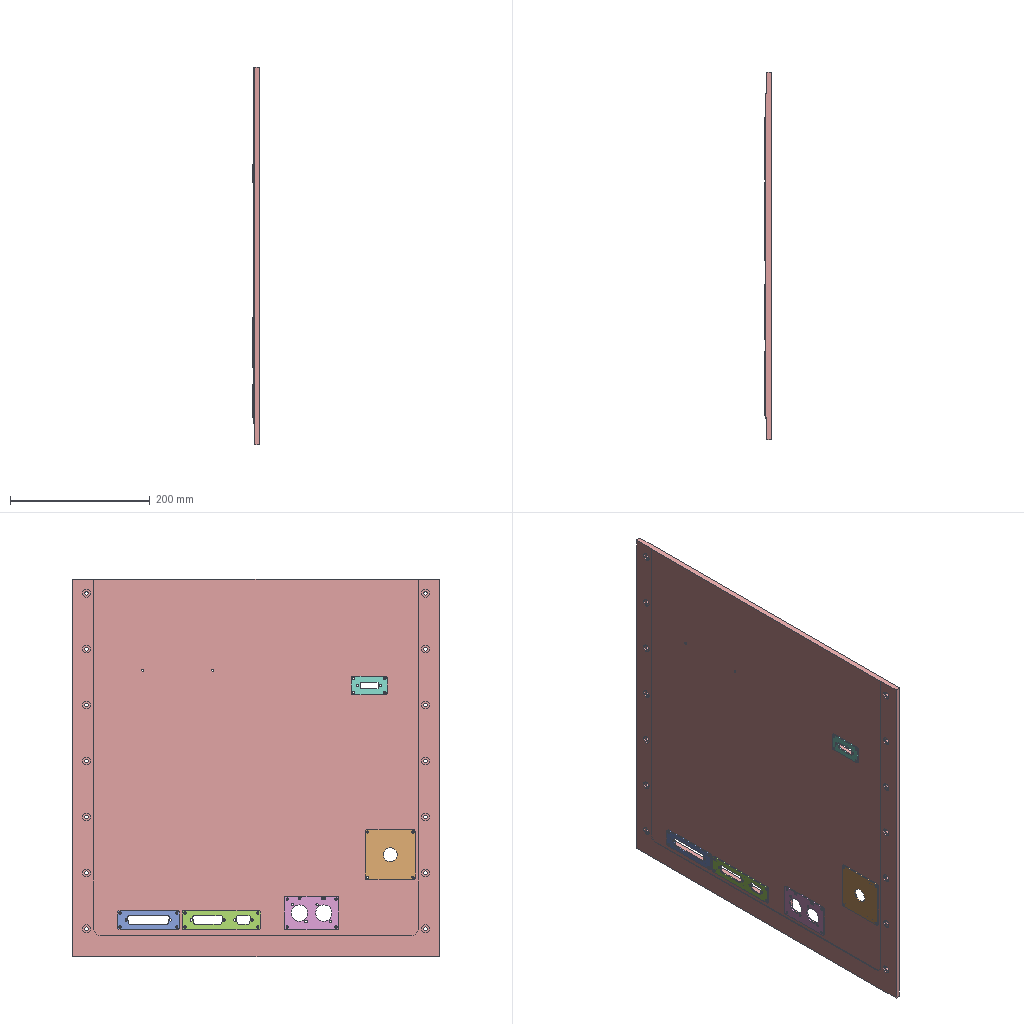Assembly | SolidWorks | 6 different items | 6 placed | box 10 x 525 x 540 mm
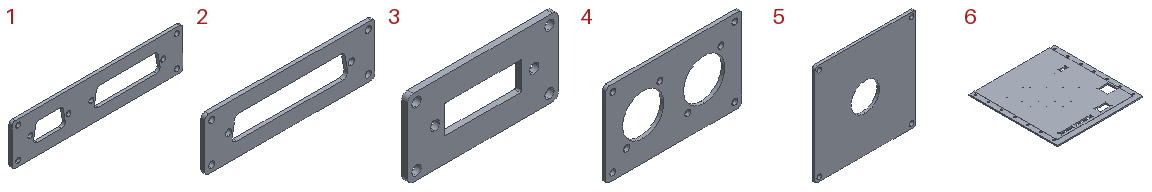Parts list (item | quantity | size | volume | features):
1 | x1 | 112 x 2 x 27 mm | 4446 mm3 | features Cut 1, Extrusion 1, Fillet 1, ICE 1
2 | x1 | 88 x 2 x 27 mm | 3241 mm3 | features ICE 3, Extrusion 1, Fillet 1, HoleWzd 1
3 | x1 | 51 x 2 x 26 mm | 2048 mm3 | features Cut 1, Extrusion 1, Fillet 1
4 | x1 | 78 x 2 x 48 mm | 5579 mm3 | features MoveFace 2, Cut 1, Extrusion 1, Fillet 1, ICE 1, LPattern 1
5 | x1 | 71 x 2 x 71 mm | 9382 mm3 | features Extrusion 1, ICE 1
6 | x1 | 525 x 540 x 8 mm | 2142455 mm3 | features HoleWzd 6, MoveFace 5, BaseBody 1, Fillet 1, ICE 1
Mates (type | each side: item.copy, entity, surface, feature):
Coincident | 6.1 face plane Imported1 | 2.1 face plane Boss-Extrude1
Concentric | 6.1 face cylinder M3 Tapped Hole1 | 2.1 face cylinder Cut-Extrude1 | 2 times
Coincident | 6.1 face plane Imported1 | 1.1 face plane Boss-Extrude1
Concentric | 6.1 face cylinder M3 Tapped Hole1 | 1.1 face cylinder Cut-Extrude1 | 2 times
Coincident | 6.1 face plane Imported1 | 4.1 face plane Boss-Extrude1
Coincident | 6.1 face plane Imported1 | 3.1 face plane Boss-Extrude1
Concentric | 6.1 face cylinder M3 Tapped Hole3 | 3.1 face cylinder Boss-Extrude1 | 2 times
Coincident | 6.1 face plane Imported1 | 5.1 face plane Boss-Extrude1
Concentric | 6.1 face cylinder M3 Tapped Hole4 | 5.1 face cylinder Boss-Extrude1 | 2 times
Concentric | 6.1 face cylinder M3 Tapped Hole2 | 4.1 face cylinder Boss-Extrude1 | 2 times